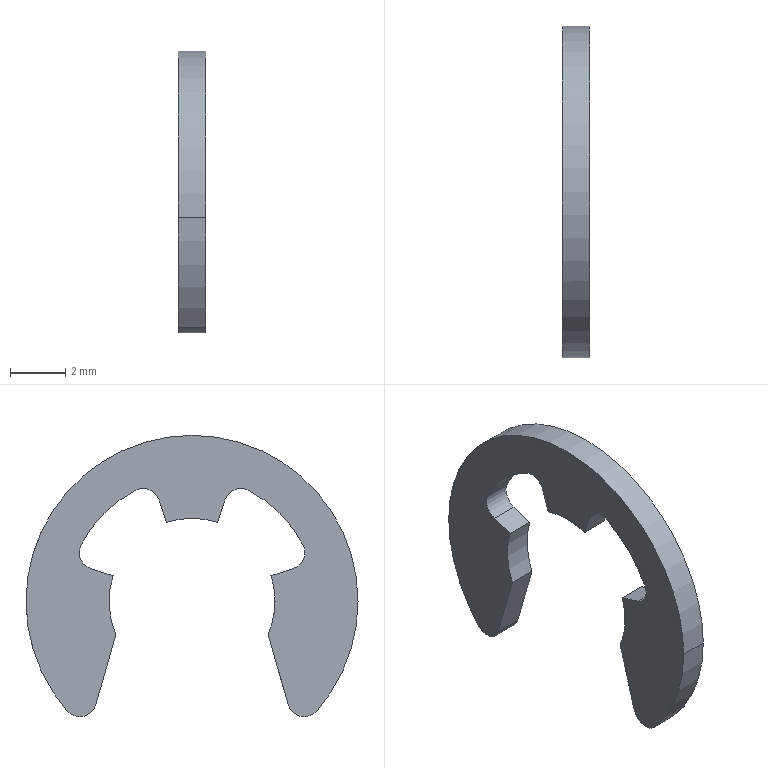Part | SolidWorks | features BaseBody 1 | 1 solid | 24 faces | box 1.012 x 12.001 x 10.168 mm | volume 51.882 mm3 | cylinder 16 | plane 8 | commonest cylinder face diameters 1.2 x7 6 x4 12 x3 9 x2
STEP:
#1=CARTESIAN_POINT('',(349.387,461.892,108.681));
#2=VERTEX_POINT('',#1);
#3=CARTESIAN_POINT('',(349.387,461.956,108.952));
#4=VERTEX_POINT('',#3);
#5=CARTESIAN_POINT('',(349.386,462.492,108.681));
#6=DIRECTION('',(-1.,-0.0009599,0.));
#7=DIRECTION('',(0.0009599,-1.,0.));
#8=AXIS2_PLACEMENT_3D('',#5,#6,#7);
#9=CIRCLE('',#8,0.6);
#10=EDGE_CURVE('',#2,#4,#9,.T.);
#11=ORIENTED_EDGE('',*,*,#10,.F.);
#12=CARTESIAN_POINT('',(348.387,461.891,108.681));
#13=VERTEX_POINT('',#12);
#14=CARTESIAN_POINT('',(349.387,461.892,108.681));
#15=DIRECTION('',(-1.,-0.0009599,0.));
#16=VECTOR('',#15,1000.);
#17=LINE('',#14,#16);
#18=EDGE_CURVE('',#2,#13,#17,.T.);
#19=ORIENTED_EDGE('',*,*,#18,.T.);
#20=CARTESIAN_POINT('',(348.387,461.955,108.952));
#21=VERTEX_POINT('',#20);
#22=CARTESIAN_POINT('',(348.386,462.491,108.681));
#23=DIRECTION('',(1.,0.0009599,0.));
#24=DIRECTION('',(0.0009599,-1.,0.));
#25=AXIS2_PLACEMENT_3D('',#22,#23,#24);
#26=CIRCLE('',#25,0.6);
#27=EDGE_CURVE('',#21,#13,#26,.T.);
#28=ORIENTED_EDGE('',*,*,#27,.F.);
#29=CARTESIAN_POINT('',(348.387,461.955,108.952));
#30=DIRECTION('',(1.,0.0009599,0.));
#31=VECTOR('',#30,1000.);
#32=LINE('',#29,#31);
#33=EDGE_CURVE('',#21,#4,#32,.T.);
#34=ORIENTED_EDGE('',*,*,#33,.T.);
#35=EDGE_LOOP('',(#11,#19,#28,#34));
#36=FACE_OUTER_BOUND('',#35,.T.);
#37=CARTESIAN_POINT('',(349.386,462.492,108.681));
#38=DIRECTION('',(-1.,-0.0009599,0.));
#39=DIRECTION('',(0.0009599,-1.,0.));
#40=AXIS2_PLACEMENT_3D('',#37,#38,#39);
#41=CYLINDRICAL_SURFACE('',#40,0.6);
#42=ADVANCED_FACE('',(#36),#41,.F.);
#43=CARTESIAN_POINT('',(349.386,462.971,106.919));
#44=VERTEX_POINT('',#43);
#45=CARTESIAN_POINT('',(349.385,463.118,107.846));
#46=VERTEX_POINT('',#45);
#47=CARTESIAN_POINT('',(349.383,465.971,106.919));
#48=DIRECTION('',(-1.,-0.0009599,0.));
#49=DIRECTION('',(0.0008799,-0.9167,-0.3997));
#50=AXIS2_PLACEMENT_3D('',#47,#48,#49);
#51=CIRCLE('',#50,3.);
#52=EDGE_CURVE('',#44,#46,#51,.T.);
#53=ORIENTED_EDGE('',*,*,#52,.F.);
#54=CARTESIAN_POINT('',(348.386,462.97,106.919));
#55=VERTEX_POINT('',#54);
#56=CARTESIAN_POINT('',(349.386,462.971,106.919));
#57=DIRECTION('',(-1.,-0.0009599,0.));
#58=VECTOR('',#57,1000.);
#59=LINE('',#56,#58);
#60=EDGE_CURVE('',#44,#55,#59,.T.);
#61=ORIENTED_EDGE('',*,*,#60,.T.);
#62=CARTESIAN_POINT('',(348.385,463.117,107.846));
#63=VERTEX_POINT('',#62);
#64=CARTESIAN_POINT('',(348.383,465.97,106.919));
#65=DIRECTION('',(1.,0.0009599,0.));
#66=DIRECTION('',(0.0009129,-0.9511,0.309));
#67=AXIS2_PLACEMENT_3D('',#64,#65,#66);
#68=CIRCLE('',#67,3.);
#69=EDGE_CURVE('',#63,#55,#68,.T.);
#70=ORIENTED_EDGE('',*,*,#69,.F.);
#71=CARTESIAN_POINT('',(348.385,463.117,107.846));
#72=DIRECTION('',(1.,0.0009599,0.));
#73=VECTOR('',#72,1000.);
#74=LINE('',#71,#73);
#75=EDGE_CURVE('',#63,#46,#74,.T.);
#76=ORIENTED_EDGE('',*,*,#75,.T.);
#77=EDGE_LOOP('',(#53,#61,#70,#76));
#78=FACE_OUTER_BOUND('',#77,.T.);
#79=CARTESIAN_POINT('',(349.383,465.971,106.919));
#80=DIRECTION('',(-1.,-0.0009599,0.));
#81=DIRECTION('',(0.0009599,-1.,0.));
#82=AXIS2_PLACEMENT_3D('',#79,#80,#81);
#83=CYLINDRICAL_SURFACE('',#82,3.);
#84=ADVANCED_FACE('',(#78),#83,.F.);
#85=CARTESIAN_POINT('',(349.377,471.971,106.919));
#86=VERTEX_POINT('',#85);
#87=CARTESIAN_POINT('',(349.388,459.971,106.919));
#88=VERTEX_POINT('',#87);
#89=CARTESIAN_POINT('',(349.383,465.971,106.919));
#90=DIRECTION('',(1.,0.0009599,0.));
#91=DIRECTION('',(-0.0007205,0.7506,-0.6607));
#92=AXIS2_PLACEMENT_3D('',#89,#90,#91);
#93=CIRCLE('',#92,6.);
#94=EDGE_CURVE('',#86,#88,#93,.T.);
#95=ORIENTED_EDGE('',*,*,#94,.F.);
#96=CARTESIAN_POINT('',(348.377,471.97,106.919));
#97=VERTEX_POINT('',#96);
#98=CARTESIAN_POINT('',(349.377,471.971,106.919));
#99=DIRECTION('',(-1.,-0.0009599,0.));
#100=VECTOR('',#99,1000.);
#101=LINE('',#98,#100);
#102=EDGE_CURVE('',#86,#97,#101,.T.);
#103=ORIENTED_EDGE('',*,*,#102,.T.);
#104=CARTESIAN_POINT('',(348.388,459.97,106.919));
#105=VERTEX_POINT('',#104);
#106=CARTESIAN_POINT('',(348.383,465.97,106.919));
#107=DIRECTION('',(-1.,-0.0009599,0.));
#108=DIRECTION('',(0.0007205,-0.7506,-0.6607));
#109=AXIS2_PLACEMENT_3D('',#106,#107,#108);
#110=CIRCLE('',#109,6.);
#111=EDGE_CURVE('',#105,#97,#110,.T.);
#112=ORIENTED_EDGE('',*,*,#111,.F.);
#113=CARTESIAN_POINT('',(349.388,459.971,106.919));
#114=DIRECTION('',(-1.,-0.0009599,0.));
#115=VECTOR('',#114,1000.);
#116=LINE('',#113,#115);
#117=EDGE_CURVE('',#88,#105,#116,.T.);
#118=ORIENTED_EDGE('',*,*,#117,.F.);
#119=EDGE_LOOP('',(#95,#103,#112,#118));
#120=FACE_OUTER_BOUND('',#119,.T.);
#121=CARTESIAN_POINT('',(349.383,465.971,106.919));
#122=DIRECTION('',(-1.,-0.0009599,0.));
#123=DIRECTION('',(0.0009599,-1.,0.));
#124=AXIS2_PLACEMENT_3D('',#121,#122,#123);
#125=CYLINDRICAL_SURFACE('',#124,6.);
#126=ADVANCED_FACE('',(#120),#125,.T.);
#127=CARTESIAN_POINT('',(349.387,461.467,102.955));
#128=VERTEX_POINT('',#127);
#129=CARTESIAN_POINT('',(349.383,465.971,106.919));
#130=DIRECTION('',(1.,0.0009599,0.));
#131=DIRECTION('',(-0.0007205,0.7506,-0.6607));
#132=AXIS2_PLACEMENT_3D('',#129,#130,#131);
#133=CIRCLE('',#132,6.);
#134=EDGE_CURVE('',#88,#128,#133,.T.);
#135=ORIENTED_EDGE('',*,*,#134,.F.);
#136=ORIENTED_EDGE('',*,*,#117,.T.);
#137=CARTESIAN_POINT('',(348.387,461.466,102.955));
#138=VERTEX_POINT('',#137);
#139=CARTESIAN_POINT('',(348.383,465.97,106.919));
#140=DIRECTION('',(-1.,-0.0009599,0.));
#141=DIRECTION('',(0.0007205,-0.7506,-0.6607));
#142=AXIS2_PLACEMENT_3D('',#139,#140,#141);
#143=CIRCLE('',#142,6.);
#144=EDGE_CURVE('',#138,#105,#143,.T.);
#145=ORIENTED_EDGE('',*,*,#144,.F.);
#146=CARTESIAN_POINT('',(348.387,461.466,102.955));
#147=DIRECTION('',(1.,0.0009599,0.));
#148=VECTOR('',#147,1000.);
#149=LINE('',#146,#148);
#150=EDGE_CURVE('',#138,#128,#149,.T.);
#151=ORIENTED_EDGE('',*,*,#150,.T.);
#152=EDGE_LOOP('',(#135,#136,#145,#151));
#153=FACE_OUTER_BOUND('',#152,.T.);
#154=CARTESIAN_POINT('',(349.383,465.971,106.919));
#155=DIRECTION('',(-1.,-0.0009599,0.));
#156=DIRECTION('',(0.0009599,-1.,0.));
#157=AXIS2_PLACEMENT_3D('',#154,#155,#156);
#158=CYLINDRICAL_SURFACE('',#157,6.);
#159=ADVANCED_FACE('',(#153),#158,.T.);
#160=CARTESIAN_POINT('',(348.385,463.938,110.934));
#161=VERTEX_POINT('',#160);
#162=CARTESIAN_POINT('',(349.385,463.939,110.934));
#163=VERTEX_POINT('',#162);
#164=CARTESIAN_POINT('',(348.385,463.938,110.934));
#165=DIRECTION('',(1.,0.0009599,0.));
#166=VECTOR('',#165,1000.);
#167=LINE('',#164,#166);
#168=EDGE_CURVE('',#161,#163,#167,.T.);
#169=ORIENTED_EDGE('',*,*,#168,.T.);
#170=CARTESIAN_POINT('',(349.383,465.971,106.919));
#171=DIRECTION('',(-1.,-0.0009599,0.));
#172=DIRECTION('',(0.0008564,-0.8922,0.4517));
#173=AXIS2_PLACEMENT_3D('',#170,#171,#172);
#174=CIRCLE('',#173,4.5);
#175=EDGE_CURVE('',#4,#163,#174,.T.);
#176=ORIENTED_EDGE('',*,*,#175,.F.);
#177=ORIENTED_EDGE('',*,*,#33,.F.);
#178=CARTESIAN_POINT('',(348.383,465.97,106.919));
#179=DIRECTION('',(1.,0.0009599,0.));
#180=DIRECTION('',(0.0004335,-0.4517,0.8922));
#181=AXIS2_PLACEMENT_3D('',#178,#179,#180);
#182=CIRCLE('',#181,4.5);
#183=EDGE_CURVE('',#161,#21,#182,.T.);
#184=ORIENTED_EDGE('',*,*,#183,.F.);
#185=EDGE_LOOP('',(#169,#176,#177,#184));
#186=FACE_OUTER_BOUND('',#185,.T.);
#187=CARTESIAN_POINT('',(349.383,465.971,106.919));
#188=DIRECTION('',(-1.,-0.0009599,0.));
#189=DIRECTION('',(0.0009599,-1.,0.));
#190=AXIS2_PLACEMENT_3D('',#187,#188,#189);
#191=CYLINDRICAL_SURFACE('',#190,4.5);
#192=ADVANCED_FACE('',(#186),#191,.F.);
#193=CARTESIAN_POINT('',(348.384,464.779,110.584));
#194=VERTEX_POINT('',#193);
#195=CARTESIAN_POINT('',(349.384,464.78,110.584));
#196=VERTEX_POINT('',#195);
#197=CARTESIAN_POINT('',(348.384,464.779,110.584));
#198=DIRECTION('',(1.,0.0009599,0.));
#199=VECTOR('',#198,1000.);
#200=LINE('',#197,#199);
#201=EDGE_CURVE('',#194,#196,#200,.T.);
#202=ORIENTED_EDGE('',*,*,#201,.T.);
#203=CARTESIAN_POINT('',(349.384,464.21,110.399));
#204=DIRECTION('',(-1.,-0.0009599,0.));
#205=DIRECTION('',(0.0004335,-0.4517,0.8922));
#206=AXIS2_PLACEMENT_3D('',#203,#204,#205);
#207=CIRCLE('',#206,0.6);
#208=EDGE_CURVE('',#163,#196,#207,.T.);
#209=ORIENTED_EDGE('',*,*,#208,.F.);
#210=ORIENTED_EDGE('',*,*,#168,.F.);
#211=CARTESIAN_POINT('',(348.384,464.209,110.399));
#212=DIRECTION('',(1.,0.0009599,0.));
#213=DIRECTION('',(-0.0009129,0.9511,0.309));
#214=AXIS2_PLACEMENT_3D('',#211,#212,#213);
#215=CIRCLE('',#214,0.6);
#216=EDGE_CURVE('',#194,#161,#215,.T.);
#217=ORIENTED_EDGE('',*,*,#216,.F.);
#218=EDGE_LOOP('',(#202,#209,#210,#217));
#219=FACE_OUTER_BOUND('',#218,.T.);
#220=CARTESIAN_POINT('',(349.384,464.21,110.399));
#221=DIRECTION('',(-1.,-0.0009599,0.));
#222=DIRECTION('',(0.0009599,-1.,0.));
#223=AXIS2_PLACEMENT_3D('',#220,#221,#222);
#224=CYLINDRICAL_SURFACE('',#223,0.6);
#225=ADVANCED_FACE('',(#219),#224,.F.);
#226=CARTESIAN_POINT('',(349.384,465.044,109.772));
#227=VERTEX_POINT('',#226);
#228=CARTESIAN_POINT('',(348.384,465.043,109.772));
#229=VERTEX_POINT('',#228);
#230=CARTESIAN_POINT('',(349.384,465.044,109.772));
#231=DIRECTION('',(-1.,-0.0009599,0.));
#232=VECTOR('',#231,1000.);
#233=LINE('',#230,#232);
#234=EDGE_CURVE('',#227,#229,#233,.T.);
#235=ORIENTED_EDGE('',*,*,#234,.F.);
#236=CARTESIAN_POINT('',(349.384,464.78,110.584));
#237=DIRECTION('',(-0.0002966,0.309,-0.9511));
#238=VECTOR('',#237,1000.);
#239=LINE('',#236,#238);
#240=EDGE_CURVE('',#196,#227,#239,.T.);
#241=ORIENTED_EDGE('',*,*,#240,.F.);
#242=ORIENTED_EDGE('',*,*,#201,.F.);
#243=CARTESIAN_POINT('',(348.384,465.043,109.772));
#244=DIRECTION('',(0.0002966,-0.309,0.9511));
#245=VECTOR('',#244,1000.);
#246=LINE('',#243,#245);
#247=EDGE_CURVE('',#229,#194,#246,.T.);
#248=ORIENTED_EDGE('',*,*,#247,.F.);
#249=EDGE_LOOP('',(#235,#241,#242,#248));
#250=FACE_OUTER_BOUND('',#249,.T.);
#251=CARTESIAN_POINT('',(349.384,464.78,110.584));
#252=DIRECTION('',(0.0009129,-0.9511,-0.309));
#253=DIRECTION('',(0.,0.309,-0.9511));
#254=AXIS2_PLACEMENT_3D('',#251,#252,#253);
#255=PLANE('',#254);
#256=ADVANCED_FACE('',(#250),#255,.T.);
#257=CARTESIAN_POINT('',(348.382,466.897,109.772));
#258=VERTEX_POINT('',#257);
#259=CARTESIAN_POINT('',(349.382,466.898,109.772));
#260=VERTEX_POINT('',#259);
#261=CARTESIAN_POINT('',(348.382,466.897,109.772));
#262=DIRECTION('',(1.,0.0009599,0.));
#263=VECTOR('',#262,1000.);
#264=LINE('',#261,#263);
#265=EDGE_CURVE('',#258,#260,#264,.T.);
#266=ORIENTED_EDGE('',*,*,#265,.T.);
#267=CARTESIAN_POINT('',(349.383,465.971,106.919));
#268=DIRECTION('',(-1.,-0.0009599,0.));
#269=DIRECTION('',(0.0002966,-0.309,0.9511));
#270=AXIS2_PLACEMENT_3D('',#267,#268,#269);
#271=CIRCLE('',#270,3.);
#272=EDGE_CURVE('',#227,#260,#271,.T.);
#273=ORIENTED_EDGE('',*,*,#272,.F.);
#274=ORIENTED_EDGE('',*,*,#234,.T.);
#275=CARTESIAN_POINT('',(348.383,465.97,106.919));
#276=DIRECTION('',(1.,0.0009599,0.));
#277=DIRECTION('',(-0.0002966,0.309,0.9511));
#278=AXIS2_PLACEMENT_3D('',#275,#276,#277);
#279=CIRCLE('',#278,3.);
#280=EDGE_CURVE('',#258,#229,#279,.T.);
#281=ORIENTED_EDGE('',*,*,#280,.F.);
#282=EDGE_LOOP('',(#266,#273,#274,#281));
#283=FACE_OUTER_BOUND('',#282,.T.);
#284=CARTESIAN_POINT('',(349.383,465.971,106.919));
#285=DIRECTION('',(-1.,-0.0009599,0.));
#286=DIRECTION('',(0.0009599,-1.,0.));
#287=AXIS2_PLACEMENT_3D('',#284,#285,#286);
#288=CYLINDRICAL_SURFACE('',#287,3.);
#289=ADVANCED_FACE('',(#283),#288,.F.);
#290=CARTESIAN_POINT('',(349.382,467.162,110.584));
#291=VERTEX_POINT('',#290);
#292=CARTESIAN_POINT('',(348.382,467.161,110.584));
#293=VERTEX_POINT('',#292);
#294=CARTESIAN_POINT('',(349.382,467.162,110.584));
#295=DIRECTION('',(-1.,-0.0009599,0.));
#296=VECTOR('',#295,1000.);
#297=LINE('',#294,#296);
#298=EDGE_CURVE('',#291,#293,#297,.T.);
#299=ORIENTED_EDGE('',*,*,#298,.F.);
#300=CARTESIAN_POINT('',(349.382,466.898,109.772));
#301=DIRECTION('',(-0.0002966,0.309,0.9511));
#302=VECTOR('',#301,1000.);
#303=LINE('',#300,#302);
#304=EDGE_CURVE('',#260,#291,#303,.T.);
#305=ORIENTED_EDGE('',*,*,#304,.F.);
#306=ORIENTED_EDGE('',*,*,#265,.F.);
#307=CARTESIAN_POINT('',(348.382,467.161,110.584));
#308=DIRECTION('',(0.0002966,-0.309,-0.9511));
#309=VECTOR('',#308,1000.);
#310=LINE('',#307,#309);
#311=EDGE_CURVE('',#293,#258,#310,.T.);
#312=ORIENTED_EDGE('',*,*,#311,.F.);
#313=EDGE_LOOP('',(#299,#305,#306,#312));
#314=FACE_OUTER_BOUND('',#313,.T.);
#315=CARTESIAN_POINT('',(349.382,467.162,110.584));
#316=DIRECTION('',(-0.0009129,0.9511,-0.309));
#317=DIRECTION('',(-1.,0.,0.002954));
#318=AXIS2_PLACEMENT_3D('',#315,#316,#317);
#319=PLANE('',#318);
#320=ADVANCED_FACE('',(#314),#319,.T.);
#321=CARTESIAN_POINT('',(348.381,468.003,110.934));
#322=VERTEX_POINT('',#321);
#323=CARTESIAN_POINT('',(349.381,468.004,110.934));
#324=VERTEX_POINT('',#323);
#325=CARTESIAN_POINT('',(348.381,468.003,110.934));
#326=DIRECTION('',(1.,0.0009599,0.));
#327=VECTOR('',#326,1000.);
#328=LINE('',#325,#327);
#329=EDGE_CURVE('',#322,#324,#328,.T.);
#330=ORIENTED_EDGE('',*,*,#329,.T.);
#331=CARTESIAN_POINT('',(349.381,467.733,110.399));
#332=DIRECTION('',(-1.,-0.0009599,0.));
#333=DIRECTION('',(0.0009129,-0.9511,0.309));
#334=AXIS2_PLACEMENT_3D('',#331,#332,#333);
#335=CIRCLE('',#334,0.6);
#336=EDGE_CURVE('',#291,#324,#335,.T.);
#337=ORIENTED_EDGE('',*,*,#336,.F.);
#338=ORIENTED_EDGE('',*,*,#298,.T.);
#339=CARTESIAN_POINT('',(348.381,467.732,110.399));
#340=DIRECTION('',(1.,0.0009599,0.));
#341=DIRECTION('',(-0.0004335,0.4517,0.8922));
#342=AXIS2_PLACEMENT_3D('',#339,#340,#341);
#343=CIRCLE('',#342,0.6);
#344=EDGE_CURVE('',#322,#293,#343,.T.);
#345=ORIENTED_EDGE('',*,*,#344,.F.);
#346=EDGE_LOOP('',(#330,#337,#338,#345));
#347=FACE_OUTER_BOUND('',#346,.T.);
#348=CARTESIAN_POINT('',(349.381,467.733,110.399));
#349=DIRECTION('',(-1.,-0.0009599,0.));
#350=DIRECTION('',(0.0009599,-1.,0.));
#351=AXIS2_PLACEMENT_3D('',#348,#349,#350);
#352=CYLINDRICAL_SURFACE('',#351,0.6);
#353=ADVANCED_FACE('',(#347),#352,.F.);
#354=CARTESIAN_POINT('',(348.379,469.985,108.952));
#355=VERTEX_POINT('',#354);
#356=CARTESIAN_POINT('',(349.379,469.986,108.952));
#357=VERTEX_POINT('',#356);
#358=CARTESIAN_POINT('',(348.379,469.985,108.952));
#359=DIRECTION('',(1.,0.0009599,0.));
#360=VECTOR('',#359,1000.);
#361=LINE('',#358,#360);
#362=EDGE_CURVE('',#355,#357,#361,.T.);
#363=ORIENTED_EDGE('',*,*,#362,.T.);
#364=CARTESIAN_POINT('',(349.383,465.971,106.919));
#365=DIRECTION('',(-1.,-0.0009599,0.));
#366=DIRECTION('',(-0.0004335,0.4517,0.8922));
#367=AXIS2_PLACEMENT_3D('',#364,#365,#366);
#368=CIRCLE('',#367,4.5);
#369=EDGE_CURVE('',#324,#357,#368,.T.);
#370=ORIENTED_EDGE('',*,*,#369,.F.);
#371=ORIENTED_EDGE('',*,*,#329,.F.);
#372=CARTESIAN_POINT('',(348.383,465.97,106.919));
#373=DIRECTION('',(1.,0.0009599,0.));
#374=DIRECTION('',(-0.0008564,0.8922,0.4517));
#375=AXIS2_PLACEMENT_3D('',#372,#373,#374);
#376=CIRCLE('',#375,4.5);
#377=EDGE_CURVE('',#355,#322,#376,.T.);
#378=ORIENTED_EDGE('',*,*,#377,.F.);
#379=EDGE_LOOP('',(#363,#370,#371,#378));
#380=FACE_OUTER_BOUND('',#379,.T.);
#381=CARTESIAN_POINT('',(349.383,465.971,106.919));
#382=DIRECTION('',(-1.,-0.0009599,0.));
#383=DIRECTION('',(0.0009599,-1.,0.));
#384=AXIS2_PLACEMENT_3D('',#381,#382,#383);
#385=CYLINDRICAL_SURFACE('',#384,4.5);
#386=ADVANCED_FACE('',(#380),#385,.F.);
#387=CARTESIAN_POINT('',(348.379,469.635,108.11));
#388=VERTEX_POINT('',#387);
#389=CARTESIAN_POINT('',(348.379,469.45,108.681));
#390=DIRECTION('',(1.,0.0009599,0.));
#391=DIRECTION('',(-0.0002966,0.309,-0.9511));
#392=AXIS2_PLACEMENT_3D('',#389,#390,#391);
#393=CIRCLE('',#392,0.6);
#394=EDGE_CURVE('',#388,#355,#393,.T.);
#395=ORIENTED_EDGE('',*,*,#394,.F.);
#396=CARTESIAN_POINT('',(349.379,469.636,108.11));
#397=VERTEX_POINT('',#396);
#398=CARTESIAN_POINT('',(348.379,469.635,108.11));
#399=DIRECTION('',(1.,0.0009599,0.));
#400=VECTOR('',#399,1000.);
#401=LINE('',#398,#400);
#402=EDGE_CURVE('',#388,#397,#401,.T.);
#403=ORIENTED_EDGE('',*,*,#402,.T.);
#404=CARTESIAN_POINT('',(349.379,469.451,108.681));
#405=DIRECTION('',(-1.,-0.0009599,0.));
#406=DIRECTION('',(-0.0008564,0.8922,0.4517));
#407=AXIS2_PLACEMENT_3D('',#404,#405,#406);
#408=CIRCLE('',#407,0.6);
#409=EDGE_CURVE('',#357,#397,#408,.T.);
#410=ORIENTED_EDGE('',*,*,#409,.F.);
#411=ORIENTED_EDGE('',*,*,#362,.F.);
#412=EDGE_LOOP('',(#395,#403,#410,#411));
#413=FACE_OUTER_BOUND('',#412,.T.);
#414=CARTESIAN_POINT('',(349.379,469.451,108.681));
#415=DIRECTION('',(-1.,-0.0009599,0.));
#416=DIRECTION('',(0.0009599,-1.,0.));
#417=AXIS2_PLACEMENT_3D('',#414,#415,#416);
#418=CYLINDRICAL_SURFACE('',#417,0.6);
#419=ADVANCED_FACE('',(#413),#418,.F.);
#420=CARTESIAN_POINT('',(349.38,468.824,107.846));
#421=VERTEX_POINT('',#420);
#422=CARTESIAN_POINT('',(348.38,468.823,107.846));
#423=VERTEX_POINT('',#422);
#424=CARTESIAN_POINT('',(349.38,468.824,107.846));
#425=DIRECTION('',(-1.,-0.0009599,0.));
#426=VECTOR('',#425,1000.);
#427=LINE('',#424,#426);
#428=EDGE_CURVE('',#421,#423,#427,.T.);
#429=ORIENTED_EDGE('',*,*,#428,.F.);
#430=CARTESIAN_POINT('',(349.379,469.636,108.11));
#431=DIRECTION('',(0.0009129,-0.9511,-0.309));
#432=VECTOR('',#431,1000.);
#433=LINE('',#430,#432);
#434=EDGE_CURVE('',#397,#421,#433,.T.);
#435=ORIENTED_EDGE('',*,*,#434,.F.);
#436=ORIENTED_EDGE('',*,*,#402,.F.);
#437=CARTESIAN_POINT('',(348.38,468.823,107.846));
#438=DIRECTION('',(-0.0009129,0.9511,0.309));
#439=VECTOR('',#438,1000.);
#440=LINE('',#437,#439);
#441=EDGE_CURVE('',#423,#388,#440,.T.);
#442=ORIENTED_EDGE('',*,*,#441,.F.);
#443=EDGE_LOOP('',(#429,#435,#436,#442));
#444=FACE_OUTER_BOUND('',#443,.T.);
#445=CARTESIAN_POINT('',(349.38,468.824,107.846));
#446=DIRECTION('',(0.0002966,-0.309,0.9511));
#447=DIRECTION('',(-1.,-0.0009599,0.));
#448=AXIS2_PLACEMENT_3D('',#445,#446,#447);
#449=PLANE('',#448);
#450=ADVANCED_FACE('',(#444),#449,.T.);
#451=CARTESIAN_POINT('',(348.38,468.72,105.72));
#452=VERTEX_POINT('',#451);
#453=CARTESIAN_POINT('',(349.38,468.721,105.72));
#454=VERTEX_POINT('',#453);
#455=CARTESIAN_POINT('',(348.38,468.72,105.72));
#456=DIRECTION('',(1.,0.0009599,0.));
#457=VECTOR('',#456,1000.);
#458=LINE('',#455,#457);
#459=EDGE_CURVE('',#452,#454,#458,.T.);
#460=ORIENTED_EDGE('',*,*,#459,.T.);
#461=CARTESIAN_POINT('',(349.383,465.971,106.919));
#462=DIRECTION('',(-1.,-0.0009599,0.));
#463=DIRECTION('',(-0.0009129,0.9511,0.309));
#464=AXIS2_PLACEMENT_3D('',#461,#462,#463);
#465=CIRCLE('',#464,3.);
#466=EDGE_CURVE('',#421,#454,#465,.T.);
#467=ORIENTED_EDGE('',*,*,#466,.F.);
#468=ORIENTED_EDGE('',*,*,#428,.T.);
#469=CARTESIAN_POINT('',(348.383,465.97,106.919));
#470=DIRECTION('',(1.,0.0009599,0.));
#471=DIRECTION('',(-0.0008799,0.9167,-0.3997));
#472=AXIS2_PLACEMENT_3D('',#469,#470,#471);
#473=CIRCLE('',#472,3.);
#474=EDGE_CURVE('',#452,#423,#473,.T.);
#475=ORIENTED_EDGE('',*,*,#474,.F.);
#476=EDGE_LOOP('',(#460,#467,#468,#475));
#477=FACE_OUTER_BOUND('',#476,.T.);
#478=CARTESIAN_POINT('',(349.383,465.971,106.919));
#479=DIRECTION('',(-1.,-0.0009599,0.));
#480=DIRECTION('',(0.0009599,-1.,0.));
#481=AXIS2_PLACEMENT_3D('',#478,#479,#480);
#482=CYLINDRICAL_SURFACE('',#481,3.);
#483=ADVANCED_FACE('',(#477),#482,.F.);
#484=CARTESIAN_POINT('',(349.379,469.448,103.186));
#485=VERTEX_POINT('',#484);
#486=CARTESIAN_POINT('',(348.379,469.447,103.186));
#487=VERTEX_POINT('',#486);
#488=CARTESIAN_POINT('',(349.379,469.448,103.186));
#489=DIRECTION('',(-1.,-0.0009599,0.));
#490=VECTOR('',#489,1000.);
#491=LINE('',#488,#490);
#492=EDGE_CURVE('',#485,#487,#491,.T.);
#493=ORIENTED_EDGE('',*,*,#492,.F.);
#494=CARTESIAN_POINT('',(349.38,468.721,105.72));
#495=DIRECTION('',(-0.0002646,0.2756,-0.9613));
#496=VECTOR('',#495,1000.);
#497=LINE('',#494,#496);
#498=EDGE_CURVE('',#454,#485,#497,.T.);
#499=ORIENTED_EDGE('',*,*,#498,.F.);
#500=ORIENTED_EDGE('',*,*,#459,.F.);
#501=CARTESIAN_POINT('',(348.379,469.447,103.186));
#502=DIRECTION('',(0.0002646,-0.2756,0.9613));
#503=VECTOR('',#502,1000.);
#504=LINE('',#501,#503);
#505=EDGE_CURVE('',#487,#452,#504,.T.);
#506=ORIENTED_EDGE('',*,*,#505,.F.);
#507=EDGE_LOOP('',(#493,#499,#500,#506));
#508=FACE_OUTER_BOUND('',#507,.T.);
#509=CARTESIAN_POINT('',(349.38,468.721,105.72));
#510=DIRECTION('',(0.0009227,-0.9613,-0.2756));
#511=DIRECTION('',(0.,0.2756,-0.9613));
#512=AXIS2_PLACEMENT_3D('',#509,#510,#511);
#513=PLANE('',#512);
#514=ADVANCED_FACE('',(#508),#513,.T.);
#515=CARTESIAN_POINT('',(348.378,470.474,102.955));
#516=VERTEX_POINT('',#515);
#517=CARTESIAN_POINT('',(349.378,470.475,102.955));
#518=VERTEX_POINT('',#517);
#519=CARTESIAN_POINT('',(348.378,470.474,102.955));
#520=DIRECTION('',(1.,0.0009599,0.));
#521=VECTOR('',#520,1000.);
#522=LINE('',#519,#521);
#523=EDGE_CURVE('',#516,#518,#522,.T.);
#524=ORIENTED_EDGE('',*,*,#523,.T.);
#525=CARTESIAN_POINT('',(349.379,470.025,103.351));
#526=DIRECTION('',(1.,0.0009599,0.));
#527=DIRECTION('',(0.0009227,-0.9613,-0.2756));
#528=AXIS2_PLACEMENT_3D('',#525,#526,#527);
#529=CIRCLE('',#528,0.6);
#530=EDGE_CURVE('',#485,#518,#529,.T.);
#531=ORIENTED_EDGE('',*,*,#530,.F.);
#532=ORIENTED_EDGE('',*,*,#492,.T.);
#533=CARTESIAN_POINT('',(348.379,470.024,103.351));
#534=DIRECTION('',(-1.,-0.0009599,0.));
#535=DIRECTION('',(-0.0007205,0.7506,-0.6607));
#536=AXIS2_PLACEMENT_3D('',#533,#534,#535);
#537=CIRCLE('',#536,0.6);
#538=EDGE_CURVE('',#516,#487,#537,.T.);
#539=ORIENTED_EDGE('',*,*,#538,.F.);
#540=EDGE_LOOP('',(#524,#531,#532,#539));
#541=FACE_OUTER_BOUND('',#540,.T.);
#542=CARTESIAN_POINT('',(349.379,470.025,103.351));
#543=DIRECTION('',(-1.,-0.0009599,0.));
#544=DIRECTION('',(0.0009599,-1.,0.));
#545=AXIS2_PLACEMENT_3D('',#542,#543,#544);
#546=CYLINDRICAL_SURFACE('',#545,0.6);
#547=ADVANCED_FACE('',(#541),#546,.T.);
#548=ORIENTED_EDGE('',*,*,#102,.F.);
#549=CARTESIAN_POINT('',(349.383,465.971,106.919));
#550=DIRECTION('',(1.,0.0009599,0.));
#551=DIRECTION('',(-0.0007205,0.7506,-0.6607));
#552=AXIS2_PLACEMENT_3D('',#549,#550,#551);
#553=CIRCLE('',#552,6.);
#554=EDGE_CURVE('',#518,#86,#553,.T.);
#555=ORIENTED_EDGE('',*,*,#554,.F.);
#556=ORIENTED_EDGE('',*,*,#523,.F.);
#557=CARTESIAN_POINT('',(348.383,465.97,106.919));
#558=DIRECTION('',(-1.,-0.0009599,0.));
#559=DIRECTION('',(0.0007205,-0.7506,-0.6607));
#560=AXIS2_PLACEMENT_3D('',#557,#558,#559);
#561=CIRCLE('',#560,6.);
#562=EDGE_CURVE('',#97,#516,#561,.T.);
#563=ORIENTED_EDGE('',*,*,#562,.F.);
#564=EDGE_LOOP('',(#548,#555,#556,#563));
#565=FACE_OUTER_BOUND('',#564,.T.);
#566=CARTESIAN_POINT('',(349.383,465.971,106.919));
#567=DIRECTION('',(-1.,-0.0009599,0.));
#568=DIRECTION('',(0.0009599,-1.,0.));
#569=AXIS2_PLACEMENT_3D('',#566,#567,#568);
#570=CYLINDRICAL_SURFACE('',#569,6.);
#571=ADVANCED_FACE('',(#565),#570,.T.);
#572=CARTESIAN_POINT('',(348.386,462.494,103.186));
#573=VERTEX_POINT('',#572);
#574=CARTESIAN_POINT('',(349.386,462.495,103.186));
#575=VERTEX_POINT('',#574);
#576=CARTESIAN_POINT('',(348.386,462.494,103.186));
#577=DIRECTION('',(1.,0.0009599,0.));
#578=VECTOR('',#577,1000.);
#579=LINE('',#576,#578);
#580=EDGE_CURVE('',#573,#575,#579,.T.);
#581=ORIENTED_EDGE('',*,*,#580,.T.);
#582=CARTESIAN_POINT('',(349.387,461.918,103.351));
#583=DIRECTION('',(1.,0.0009599,0.));
#584=DIRECTION('',(0.0007205,-0.7506,-0.6607));
#585=AXIS2_PLACEMENT_3D('',#582,#583,#584);
#586=CIRCLE('',#585,0.6);
#587=EDGE_CURVE('',#128,#575,#586,.T.);
#588=ORIENTED_EDGE('',*,*,#587,.F.);
#589=ORIENTED_EDGE('',*,*,#150,.F.);
#590=CARTESIAN_POINT('',(348.387,461.917,103.351));
#591=DIRECTION('',(-1.,-0.0009599,0.));
#592=DIRECTION('',(-0.0009227,0.9613,-0.2756));
#593=AXIS2_PLACEMENT_3D('',#590,#591,#592);
#594=CIRCLE('',#593,0.6);
#595=EDGE_CURVE('',#573,#138,#594,.T.);
#596=ORIENTED_EDGE('',*,*,#595,.F.);
#597=EDGE_LOOP('',(#581,#588,#589,#596));
#598=FACE_OUTER_BOUND('',#597,.T.);
#599=CARTESIAN_POINT('',(349.387,461.918,103.351));
#600=DIRECTION('',(-1.,-0.0009599,0.));
#601=DIRECTION('',(0.0009599,-1.,0.));
#602=AXIS2_PLACEMENT_3D('',#599,#600,#601);
#603=CYLINDRICAL_SURFACE('',#602,0.6);
#604=ADVANCED_FACE('',(#598),#603,.T.);
#605=CARTESIAN_POINT('',(349.385,463.221,105.72));
#606=VERTEX_POINT('',#605);
#607=CARTESIAN_POINT('',(348.385,463.22,105.72));
#608=VERTEX_POINT('',#607);
#609=CARTESIAN_POINT('',(349.385,463.221,105.72));
#610=DIRECTION('',(-1.,-0.0009599,0.));
#611=VECTOR('',#610,1000.);
#612=LINE('',#609,#611);
#613=EDGE_CURVE('',#606,#608,#612,.T.);
#614=ORIENTED_EDGE('',*,*,#613,.F.);
#615=CARTESIAN_POINT('',(349.386,462.495,103.186));
#616=DIRECTION('',(-0.0002646,0.2756,0.9613));
#617=VECTOR('',#616,1000.);
#618=LINE('',#615,#617);
#619=EDGE_CURVE('',#575,#606,#618,.T.);
#620=ORIENTED_EDGE('',*,*,#619,.F.);
#621=ORIENTED_EDGE('',*,*,#580,.F.);
#622=CARTESIAN_POINT('',(348.385,463.22,105.72));
#623=DIRECTION('',(0.0002646,-0.2756,-0.9613));
#624=VECTOR('',#623,1000.);
#625=LINE('',#622,#624);
#626=EDGE_CURVE('',#608,#573,#625,.T.);
#627=ORIENTED_EDGE('',*,*,#626,.F.);
#628=EDGE_LOOP('',(#614,#620,#621,#627));
#629=FACE_OUTER_BOUND('',#628,.T.);
#630=CARTESIAN_POINT('',(349.385,463.221,105.72));
#631=DIRECTION('',(-0.0009227,0.9613,-0.2756));
#632=DIRECTION('',(-1.,0.,0.003347));
#633=AXIS2_PLACEMENT_3D('',#630,#631,#632);
#634=PLANE('',#633);
#635=ADVANCED_FACE('',(#629),#634,.T.);
#636=ORIENTED_EDGE('',*,*,#60,.F.);
#637=CARTESIAN_POINT('',(349.383,465.971,106.919));
#638=DIRECTION('',(-1.,-0.0009599,0.));
#639=DIRECTION('',(0.0008799,-0.9167,-0.3997));
#640=AXIS2_PLACEMENT_3D('',#637,#638,#639);
#641=CIRCLE('',#640,3.);
#642=EDGE_CURVE('',#606,#44,#641,.T.);
#643=ORIENTED_EDGE('',*,*,#642,.F.);
#644=ORIENTED_EDGE('',*,*,#613,.T.);
#645=CARTESIAN_POINT('',(348.383,465.97,106.919));
#646=DIRECTION('',(1.,0.0009599,0.));
#647=DIRECTION('',(0.0009129,-0.9511,0.309));
#648=AXIS2_PLACEMENT_3D('',#645,#646,#647);
#649=CIRCLE('',#648,3.);
#650=EDGE_CURVE('',#55,#608,#649,.T.);
#651=ORIENTED_EDGE('',*,*,#650,.F.);
#652=EDGE_LOOP('',(#636,#643,#644,#651));
#653=FACE_OUTER_BOUND('',#652,.T.);
#654=CARTESIAN_POINT('',(349.383,465.971,106.919));
#655=DIRECTION('',(-1.,-0.0009599,0.));
#656=DIRECTION('',(0.0009599,-1.,0.));
#657=AXIS2_PLACEMENT_3D('',#654,#655,#656);
#658=CYLINDRICAL_SURFACE('',#657,3.);
#659=ADVANCED_FACE('',(#653),#658,.F.);
#660=CARTESIAN_POINT('',(349.386,462.306,108.11));
#661=VERTEX_POINT('',#660);
#662=CARTESIAN_POINT('',(348.386,462.305,108.11));
#663=VERTEX_POINT('',#662);
#664=CARTESIAN_POINT('',(349.386,462.306,108.11));
#665=DIRECTION('',(-1.,-0.0009599,0.));
#666=VECTOR('',#665,1000.);
#667=LINE('',#664,#666);
#668=EDGE_CURVE('',#661,#663,#667,.T.);
#669=ORIENTED_EDGE('',*,*,#668,.F.);
#670=CARTESIAN_POINT('',(349.385,463.118,107.846));
#671=DIRECTION('',(0.0009129,-0.9511,0.309));
#672=VECTOR('',#671,1000.);
#673=LINE('',#670,#672);
#674=EDGE_CURVE('',#46,#661,#673,.T.);
#675=ORIENTED_EDGE('',*,*,#674,.F.);
#676=ORIENTED_EDGE('',*,*,#75,.F.);
#677=CARTESIAN_POINT('',(348.386,462.305,108.11));
#678=DIRECTION('',(-0.0009129,0.9511,-0.309));
#679=VECTOR('',#678,1000.);
#680=LINE('',#677,#679);
#681=EDGE_CURVE('',#663,#63,#680,.T.);
#682=ORIENTED_EDGE('',*,*,#681,.F.);
#683=EDGE_LOOP('',(#669,#675,#676,#682));
#684=FACE_OUTER_BOUND('',#683,.T.);
#685=CARTESIAN_POINT('',(349.385,463.118,107.846));
#686=DIRECTION('',(-0.0002966,0.309,0.9511));
#687=DIRECTION('',(1.,0.0009599,0.));
#688=AXIS2_PLACEMENT_3D('',#685,#686,#687);
#689=PLANE('',#688);
#690=ADVANCED_FACE('',(#684),#689,.T.);
#691=ORIENTED_EDGE('',*,*,#175,.T.);
#692=ORIENTED_EDGE('',*,*,#208,.T.);
#693=ORIENTED_EDGE('',*,*,#240,.T.);
#694=ORIENTED_EDGE('',*,*,#272,.T.);
#695=ORIENTED_EDGE('',*,*,#304,.T.);
#696=ORIENTED_EDGE('',*,*,#336,.T.);
#697=ORIENTED_EDGE('',*,*,#369,.T.);
#698=ORIENTED_EDGE('',*,*,#409,.T.);
#699=ORIENTED_EDGE('',*,*,#434,.T.);
#700=ORIENTED_EDGE('',*,*,#466,.T.);
#701=ORIENTED_EDGE('',*,*,#498,.T.);
#702=ORIENTED_EDGE('',*,*,#530,.T.);
#703=ORIENTED_EDGE('',*,*,#554,.T.);
#704=ORIENTED_EDGE('',*,*,#94,.T.);
#705=ORIENTED_EDGE('',*,*,#134,.T.);
#706=ORIENTED_EDGE('',*,*,#587,.T.);
#707=ORIENTED_EDGE('',*,*,#619,.T.);
#708=ORIENTED_EDGE('',*,*,#642,.T.);
#709=ORIENTED_EDGE('',*,*,#52,.T.);
#710=ORIENTED_EDGE('',*,*,#674,.T.);
#711=CARTESIAN_POINT('',(349.386,462.492,108.681));
#712=DIRECTION('',(-1.,-0.0009599,0.));
#713=DIRECTION('',(0.0009599,-1.,0.));
#714=AXIS2_PLACEMENT_3D('',#711,#712,#713);
#715=CIRCLE('',#714,0.6);
#716=EDGE_CURVE('',#661,#2,#715,.T.);
#717=ORIENTED_EDGE('',*,*,#716,.T.);
#718=ORIENTED_EDGE('',*,*,#10,.T.);
#719=EDGE_LOOP('',(#691,#692,#693,#694,#695,#696,#697,#698,#699,#700,#701,#702,#703,#704,#705,#706,#707,#708,#709,#710,#717,#718));
#720=FACE_OUTER_BOUND('',#719,.T.);
#721=CARTESIAN_POINT('',(349.386,462.492,108.681));
#722=DIRECTION('',(1.,0.0009599,0.));
#723=DIRECTION('',(0.,0.,-1.));
#724=AXIS2_PLACEMENT_3D('',#721,#722,#723);
#725=PLANE('',#724);
#726=ADVANCED_FACE('',(#720),#725,.T.);
#727=ORIENTED_EDGE('',*,*,#18,.F.);
#728=ORIENTED_EDGE('',*,*,#716,.F.);
#729=ORIENTED_EDGE('',*,*,#668,.T.);
#730=CARTESIAN_POINT('',(348.386,462.491,108.681));
#731=DIRECTION('',(1.,0.0009599,0.));
#732=DIRECTION('',(0.0009599,-1.,0.));
#733=AXIS2_PLACEMENT_3D('',#730,#731,#732);
#734=CIRCLE('',#733,0.6);
#735=EDGE_CURVE('',#13,#663,#734,.T.);
#736=ORIENTED_EDGE('',*,*,#735,.F.);
#737=EDGE_LOOP('',(#727,#728,#729,#736));
#738=FACE_OUTER_BOUND('',#737,.T.);
#739=CARTESIAN_POINT('',(349.386,462.492,108.681));
#740=DIRECTION('',(-1.,-0.0009599,0.));
#741=DIRECTION('',(0.0009599,-1.,0.));
#742=AXIS2_PLACEMENT_3D('',#739,#740,#741);
#743=CYLINDRICAL_SURFACE('',#742,0.6);
#744=ADVANCED_FACE('',(#738),#743,.F.);
#745=ORIENTED_EDGE('',*,*,#27,.T.);
#746=ORIENTED_EDGE('',*,*,#735,.T.);
#747=ORIENTED_EDGE('',*,*,#681,.T.);
#748=ORIENTED_EDGE('',*,*,#69,.T.);
#749=ORIENTED_EDGE('',*,*,#650,.T.);
#750=ORIENTED_EDGE('',*,*,#626,.T.);
#751=ORIENTED_EDGE('',*,*,#595,.T.);
#752=ORIENTED_EDGE('',*,*,#144,.T.);
#753=ORIENTED_EDGE('',*,*,#111,.T.);
#754=ORIENTED_EDGE('',*,*,#562,.T.);
#755=ORIENTED_EDGE('',*,*,#538,.T.);
#756=ORIENTED_EDGE('',*,*,#505,.T.);
#757=ORIENTED_EDGE('',*,*,#474,.T.);
#758=ORIENTED_EDGE('',*,*,#441,.T.);
#759=ORIENTED_EDGE('',*,*,#394,.T.);
#760=ORIENTED_EDGE('',*,*,#377,.T.);
#761=ORIENTED_EDGE('',*,*,#344,.T.);
#762=ORIENTED_EDGE('',*,*,#311,.T.);
#763=ORIENTED_EDGE('',*,*,#280,.T.);
#764=ORIENTED_EDGE('',*,*,#247,.T.);
#765=ORIENTED_EDGE('',*,*,#216,.T.);
#766=ORIENTED_EDGE('',*,*,#183,.T.);
#767=EDGE_LOOP('',(#745,#746,#747,#748,#749,#750,#751,#752,#753,#754,#755,#756,#757,#758,#759,#760,#761,#762,#763,#764,#765,#766));
#768=FACE_OUTER_BOUND('',#767,.T.);
#769=CARTESIAN_POINT('',(348.386,462.491,108.681));
#770=DIRECTION('',(1.,0.0009599,0.));
#771=DIRECTION('',(0.,0.,-1.));
#772=AXIS2_PLACEMENT_3D('',#769,#770,#771);
#773=PLANE('',#772);
#774=ADVANCED_FACE('',(#768),#773,.F.);
#775=CLOSED_SHELL('',(#42,#84,#126,#159,#192,#225,#256,#289,#320,#353,#386,#419,#450,#483,#514,#547,#571,#604,#635,#659,#690,#726,#744,#774));
#776=MANIFOLD_SOLID_BREP('',#775);
#777=CARTESIAN_POINT('',(0.,0.,0.));
#778=DIRECTION('',(0.,0.,1.));
#779=DIRECTION('',(1.,0.,0.));
#780=AXIS2_PLACEMENT_3D('',#777,#778,#779);
#781=(LENGTH_UNIT()NAMED_UNIT(*)SI_UNIT(.MILLI.,.METRE.));
#782=UNCERTAINTY_MEASURE_WITH_UNIT(LENGTH_MEASURE(0.00001),#781,'','');
#783=(NAMED_UNIT(*)PLANE_ANGLE_UNIT()SI_UNIT($,.RADIAN.));
#784=(NAMED_UNIT(*)SI_UNIT($,.STERADIAN.)SOLID_ANGLE_UNIT());
#785=(GEOMETRIC_REPRESENTATION_CONTEXT(3)GLOBAL_UNCERTAINTY_ASSIGNED_CONTEXT((#782))GLOBAL_UNIT_ASSIGNED_CONTEXT((#781,#783,#784))REPRESENTATION_CONTEXT('',''));
#786=ADVANCED_BREP_SHAPE_REPRESENTATION('',(#776,#780),#785);